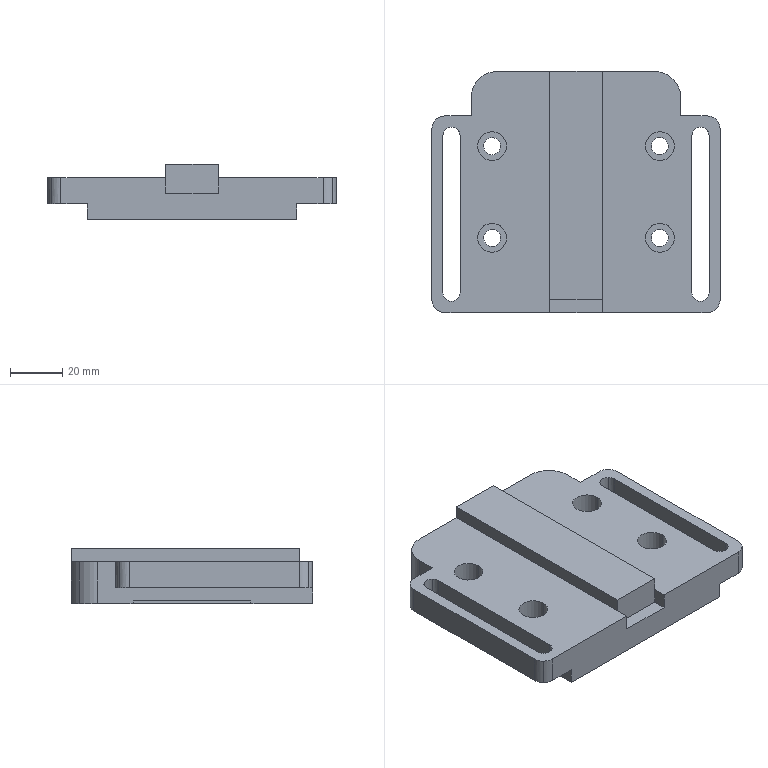Part | SolidWorks | features ICE 5, Extrusion 1 | 1 solid | 72 faces | box 110 x 92 x 21 mm | volume 133091 mm3 | plane 36 | spline 28 | cylinder 8 | commonest cylinder face diameters 11 x8